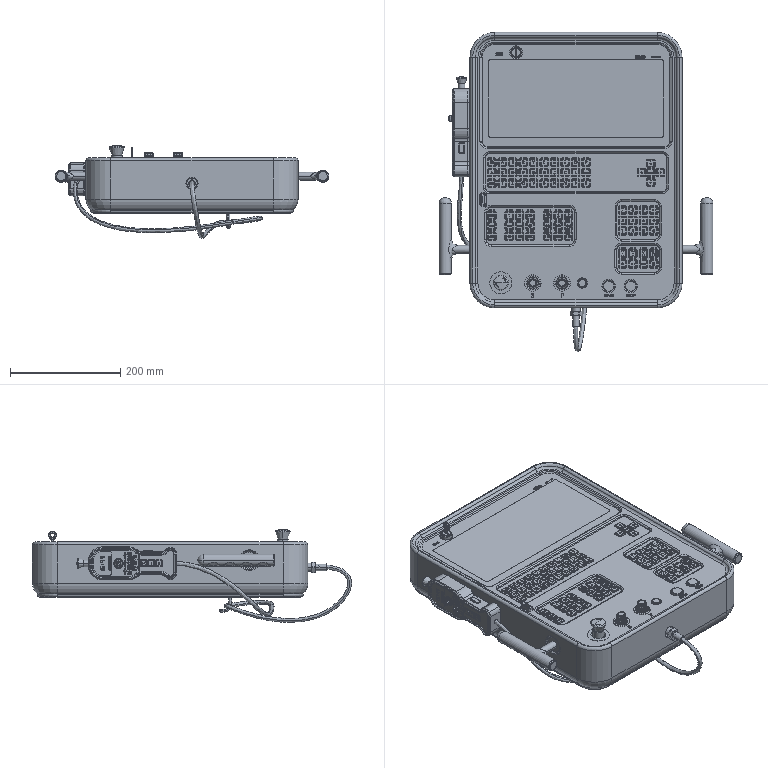Part | SolidWorks | features BaseBody 1 | 1 solid | 5898 faces | volume 17662933 mm3 | plane 2304 | cylinder 1610 | torus 975 | spline 930 | cone 66 | sphere 13 | commonest cylinder face diameters 3 x315 2.2 x308 1.2 x304 1.5 x87 1 x62 2 x54